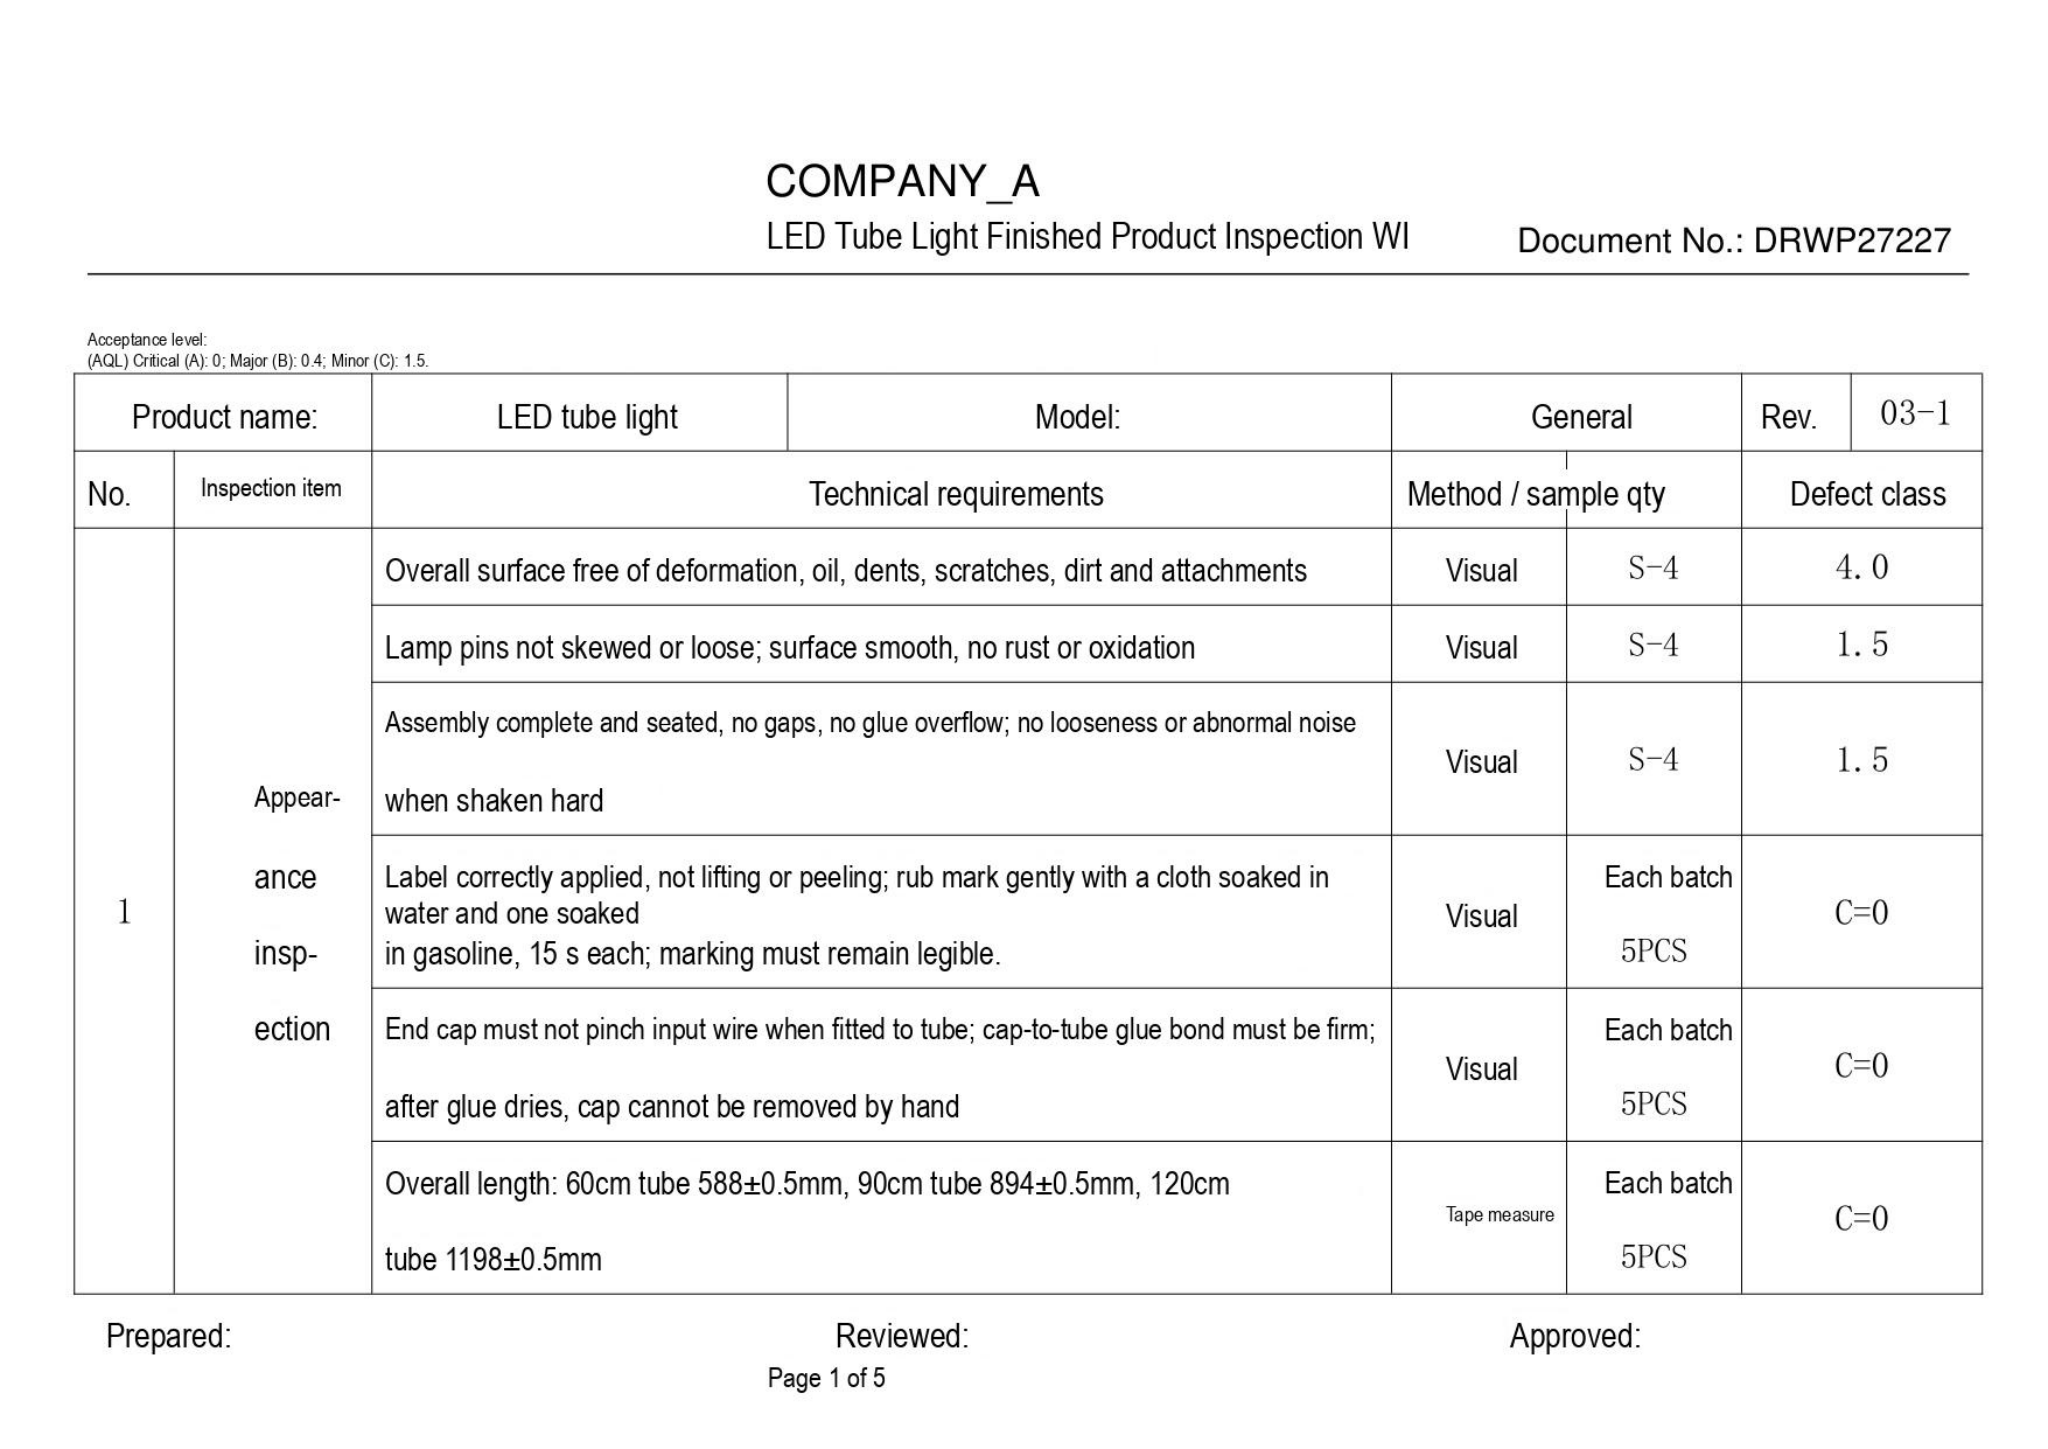COMPANY_A
LED Tube Light Finished Product Inspection WI
Document No.: DRWP27227

Acceptance level:
(AQL) Critical (A): 0; Major (B): 0.4; Minor (C): 1.5.

| Product name: | | LED tube light | Model: | General | | Rev. | 03-1 |
|---|---|---|---|---|---|---|---|
| No. | Inspection item | Technical requirements | | Method / sample qty | | Defect class | |
| 1 | Appear-ance insp-ection | Overall surface free of deformation, oil, dents, scratches, dirt and attachments | | Visual | S-4 | 4.0 | |
| | | Lamp pins not skewed or loose; surface smooth, no rust or oxidation | | Visual | S-4 | 1.5 | |
| | | Assembly complete and seated, no gaps, no glue overflow; no looseness or abnormal noise when shaken hard | | Visual | S-4 | 1.5 | |
| | | Label correctly applied, not lifting or peeling; rub mark gently with a cloth soaked in water and one soaked in gasoline, 15 s each; marking must remain legible. | | Visual | Each batch 5PCS | C=0 | |
| | | End cap must not pinch input wire when fitted to tube; cap-to-tube glue bond must be firm; after glue dries, cap cannot be removed by hand | | Visual | Each batch 5PCS | C=0 | |
| | | Overall length: 60cm tube 588±0.5mm, 90cm tube 894±0.5mm, 120cm tube 1198±0.5mm | | Tape measure | Each batch 5PCS | C=0 | |

Prepared: Reviewed: Approved:

Page 1 of 5
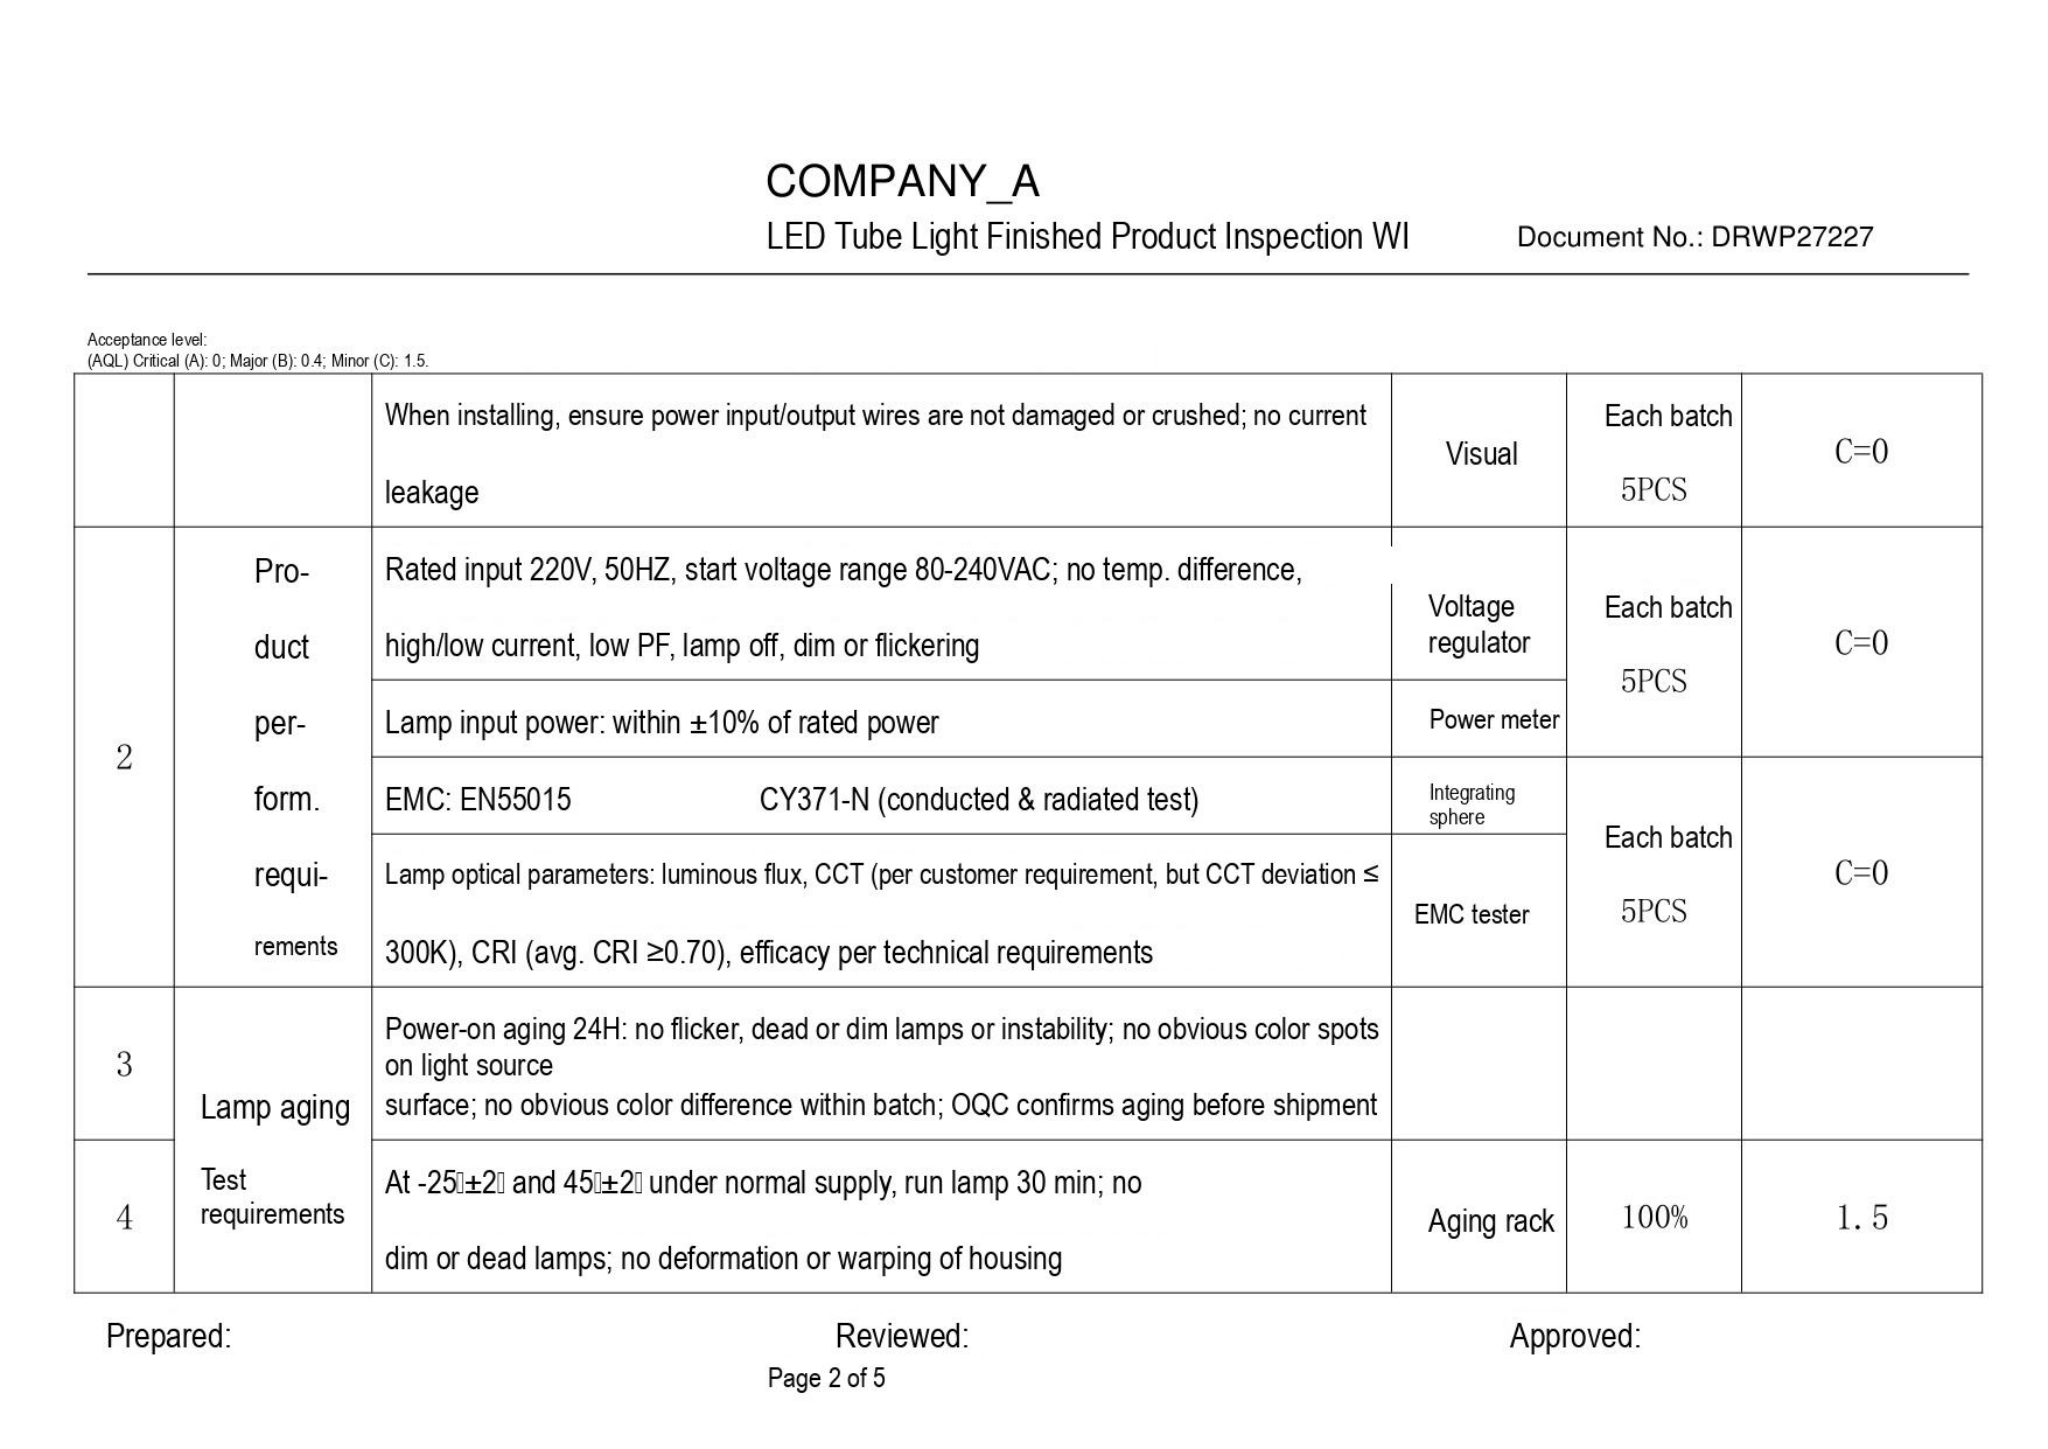COMPANY_A

LED Tube Light Finished Product Inspection WI　　Document No.: DRWP27227

Acceptance level:
(AQL) Critical (A): 0; Major (B): 0.4; Minor (C): 1.5.

| | | | | | |
|---|---|---|---|---|---|
| | | When installing, ensure power input/output wires are not damaged or crushed; no current leakage | Visual | Each batch 5PCS | C=0 |
| 2 | Pro- duct per- form. requi- rements | Rated input 220V, 50HZ, start voltage range 80-240VAC; no temp. difference, high/low current, low PF, lamp off, dim or flickering | Voltage regulator | Each batch 5PCS | C=0 |
| | | Lamp input power: within ±10% of rated power | Power meter | | |
| | | EMC: EN55015　　CY371-N (conducted & radiated test) | Integrating sphere | Each batch 5PCS | C=0 |
| | | Lamp optical parameters: luminous flux, CCT (per customer requirement, but CCT deviation ≤ 300K), CRI (avg. CRI ≥0.70), efficacy per technical requirements | EMC tester | | |
| 3 | Lamp aging | Power-on aging 24H: no flicker, dead or dim lamps or instability; no obvious color spots on light source surface; no obvious color difference within batch; OQC confirms aging before shipment | | | |
| 4 | Test requirements | At -25±2 and 45±2 under normal supply, run lamp 30 min; no dim or dead lamps; no deformation or warping of housing | Aging rack | 100% | 1.5 |

Prepared:　　Reviewed:　　Approved:

Page 2 of 5
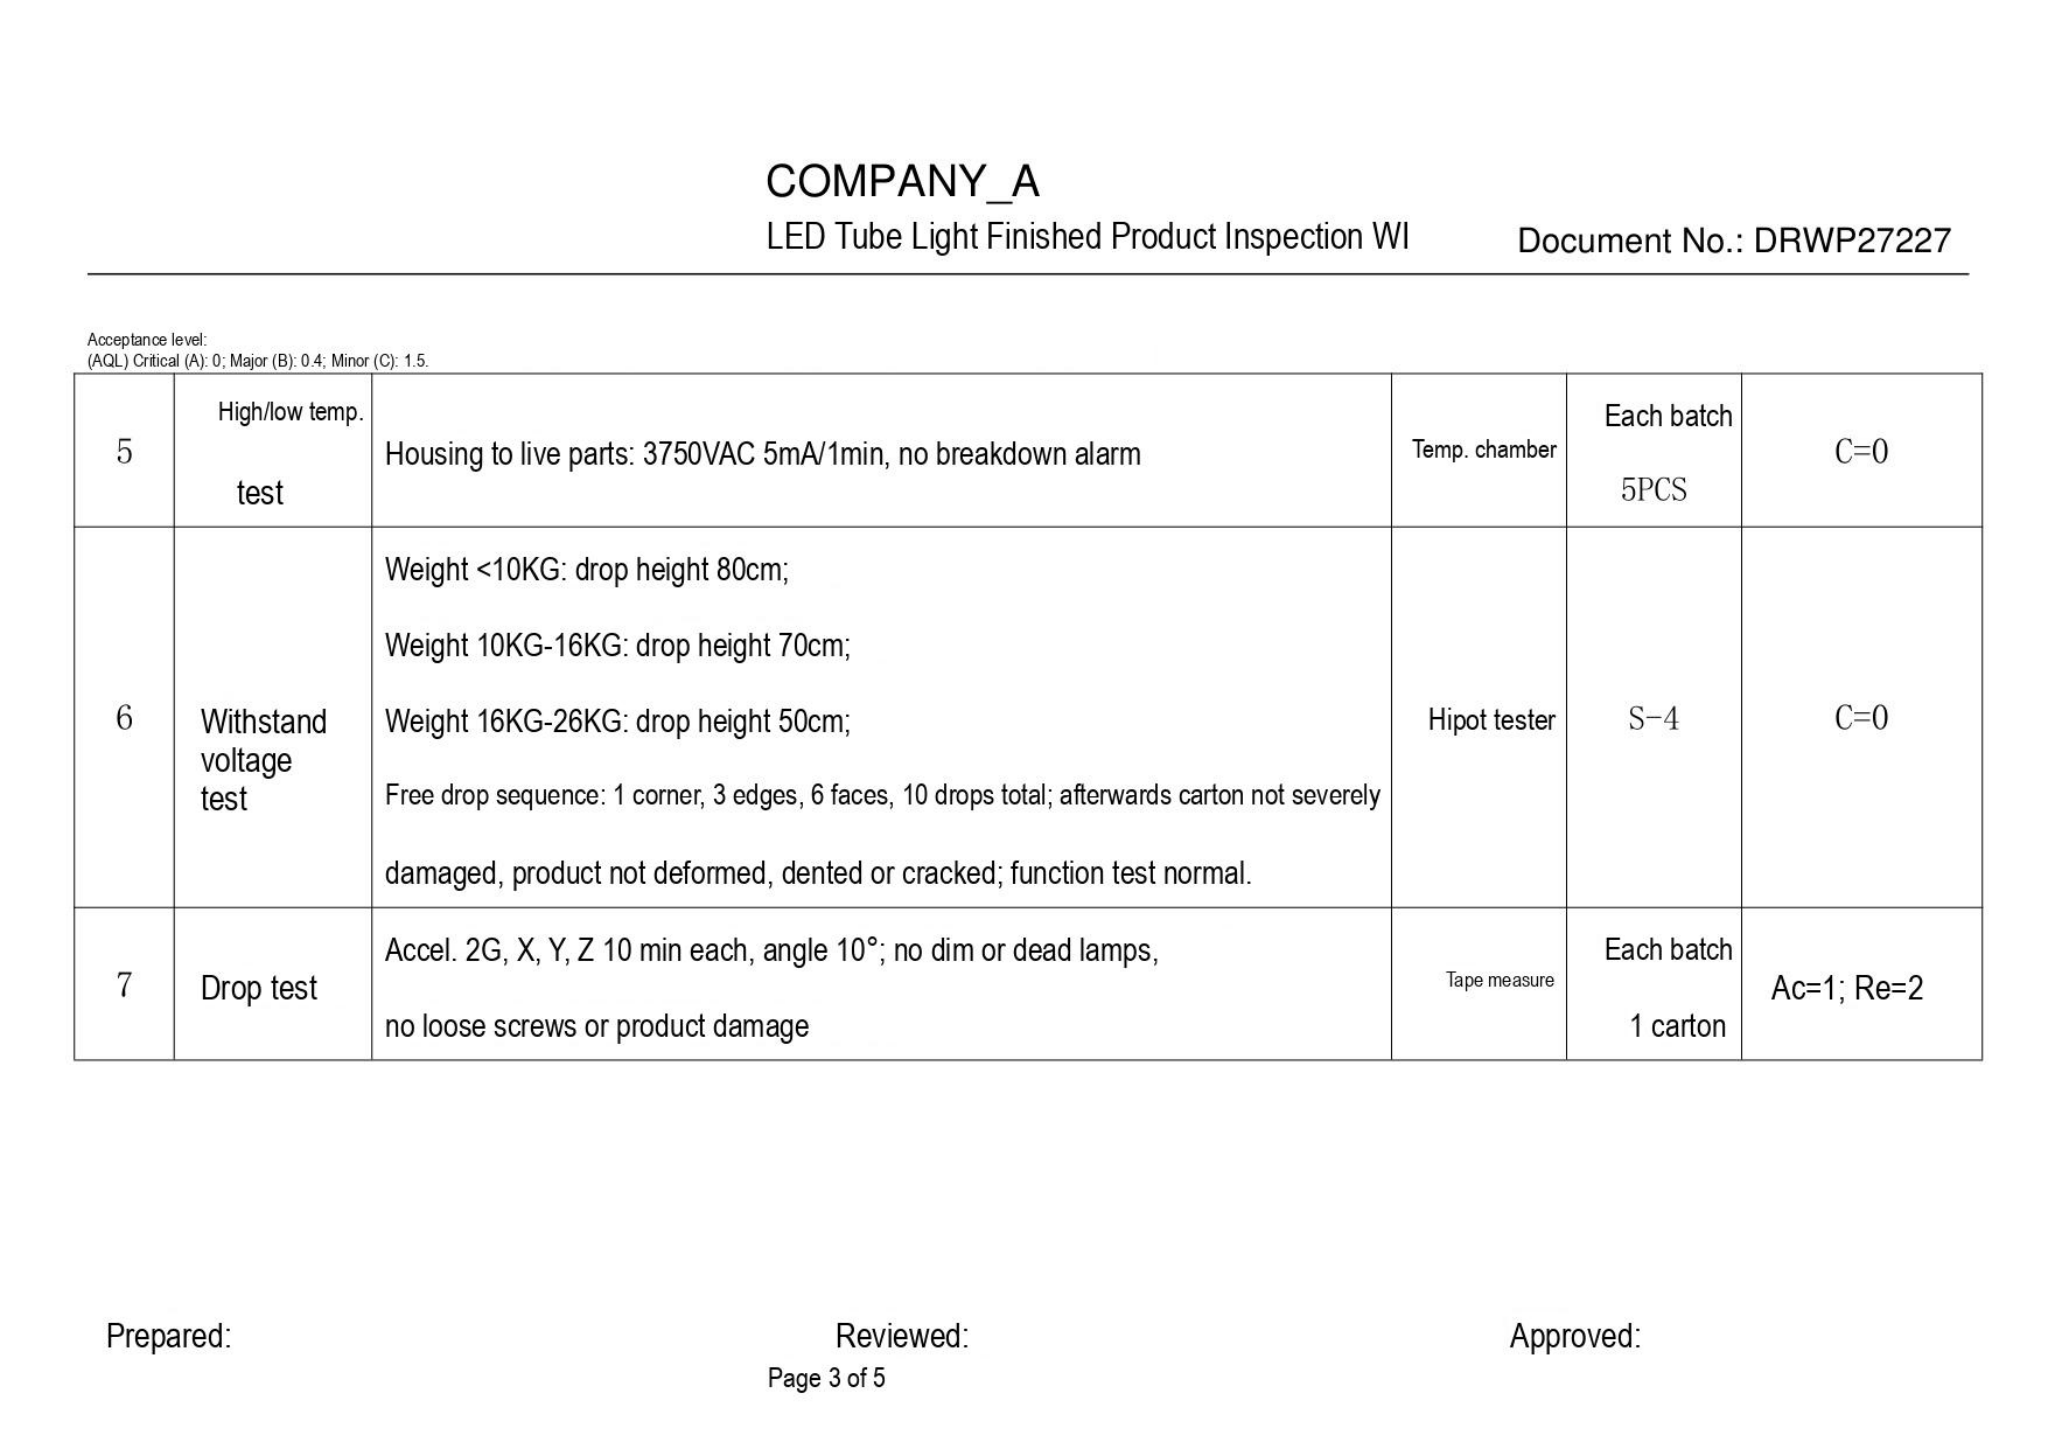COMPANY_A

LED Tube Light Finished Product Inspection WI

Document No.: DRWP27227

Acceptance level:
(AQL) Critical (A): 0; Major (B): 0.4; Minor (C): 1.5.

| 5 | High/low temp. test | Housing to live parts: 3750VAC 5mA/1min, no breakdown alarm | Temp. chamber | Each batch 5PCS | C=0 |
|---|---|---|---|---|---|
| 6 | Withstand voltage test | Weight <10KG: drop height 80cm; Weight 10KG-16KG: drop height 70cm; Weight 16KG-26KG: drop height 50cm; Free drop sequence: 1 corner, 3 edges, 6 faces, 10 drops total; afterwards carton not severely damaged, product not deformed, dented or cracked; function test normal. | Hipot tester | S-4 | C=0 |
| 7 | Drop test | Accel. 2G, X, Y, Z 10 min each, angle 10°; no dim or dead lamps, no loose screws or product damage | Tape measure | Each batch 1 carton | Ac=1; Re=2 |

Prepared:

Reviewed:

Approved:

Page 3 of 5
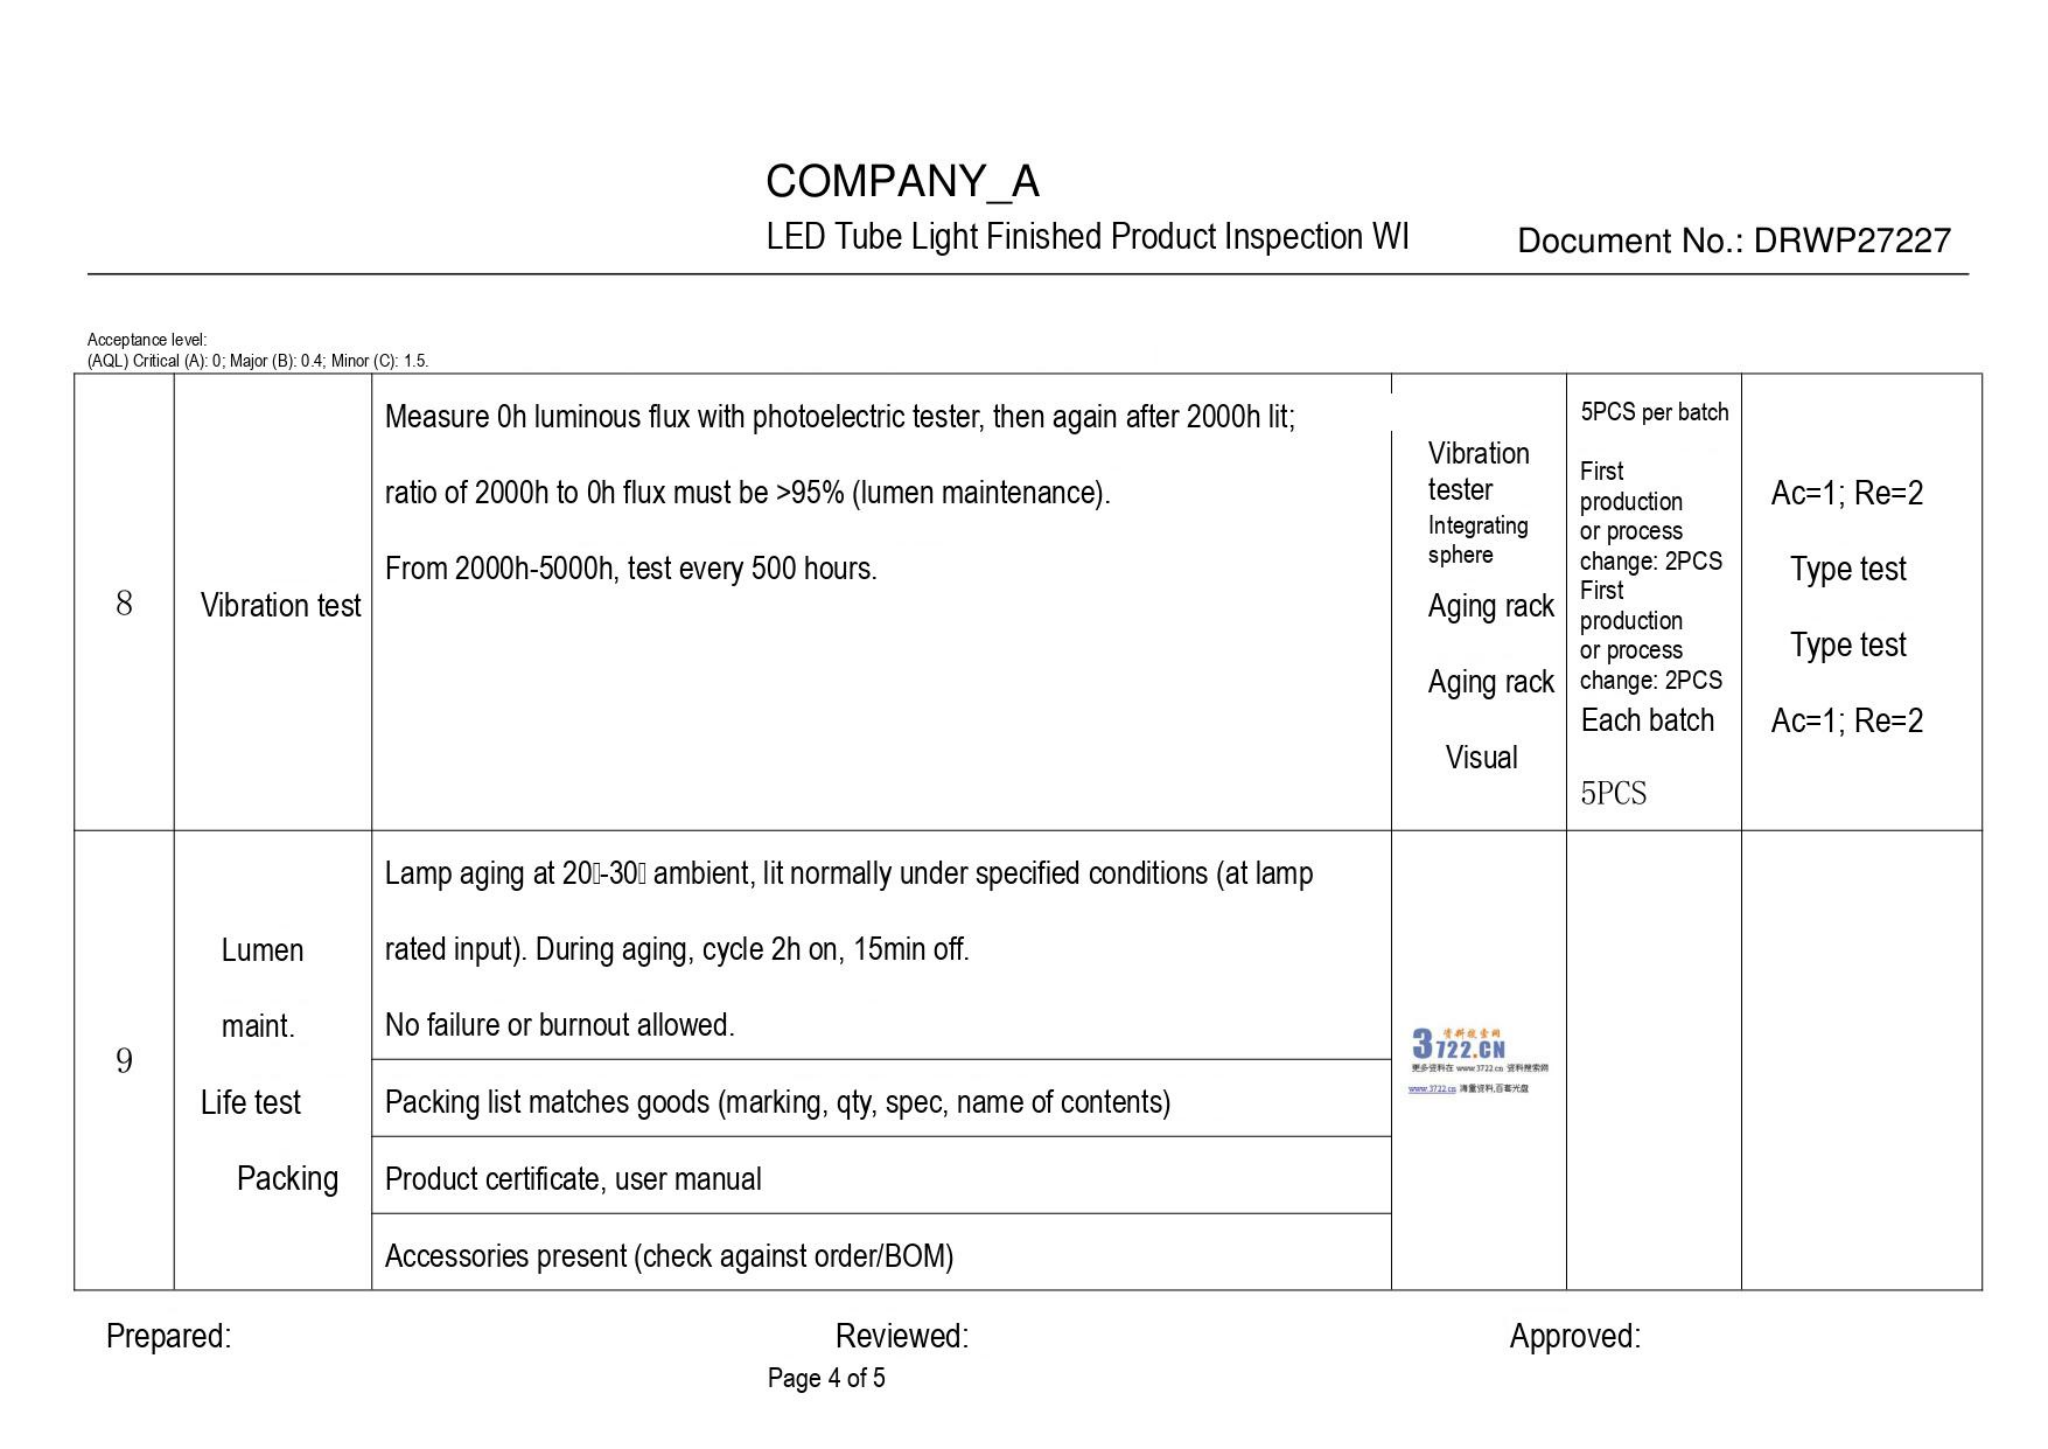COMPANY_A

LED Tube Light Finished Product Inspection WI

Document No.: DRWP27227

Acceptance level:
(AQL) Critical (A): 0; Major (B): 0.4; Minor (C): 1.5.

| | | | | | |
|---|---|---|---|---|---|
| 8 | Vibration test | Measure 0h luminous flux with photoelectric tester, then again after 2000h lit;<br>ratio of 2000h to 0h flux must be >95% (lumen maintenance).<br>From 2000h-5000h, test every 500 hours. | Vibration tester<br>Integrating sphere<br>Aging rack<br>Aging rack<br>Visual | 5PCS per batch<br>First production or process change: 2PCS<br>First production or process change: 2PCS<br>Each batch<br>5PCS | Ac=1; Re=2<br>Type test<br>Type test<br>Ac=1; Re=2 |
| 9 | Lumen maint.<br>Life test<br>Packing | Lamp aging at 20-30 ambient, lit normally under specified conditions (at lamp rated input). During aging, cycle 2h on, 15min off.<br>No failure or burnout allowed. | 3722.CN | | |
| | | Packing list matches goods (marking, qty, spec, name of contents) | | | |
| | | Product certificate, user manual | | | |
| | | Accessories present (check against order/BOM) | | | |

Prepared: Reviewed: Approved:

Page 4 of 5
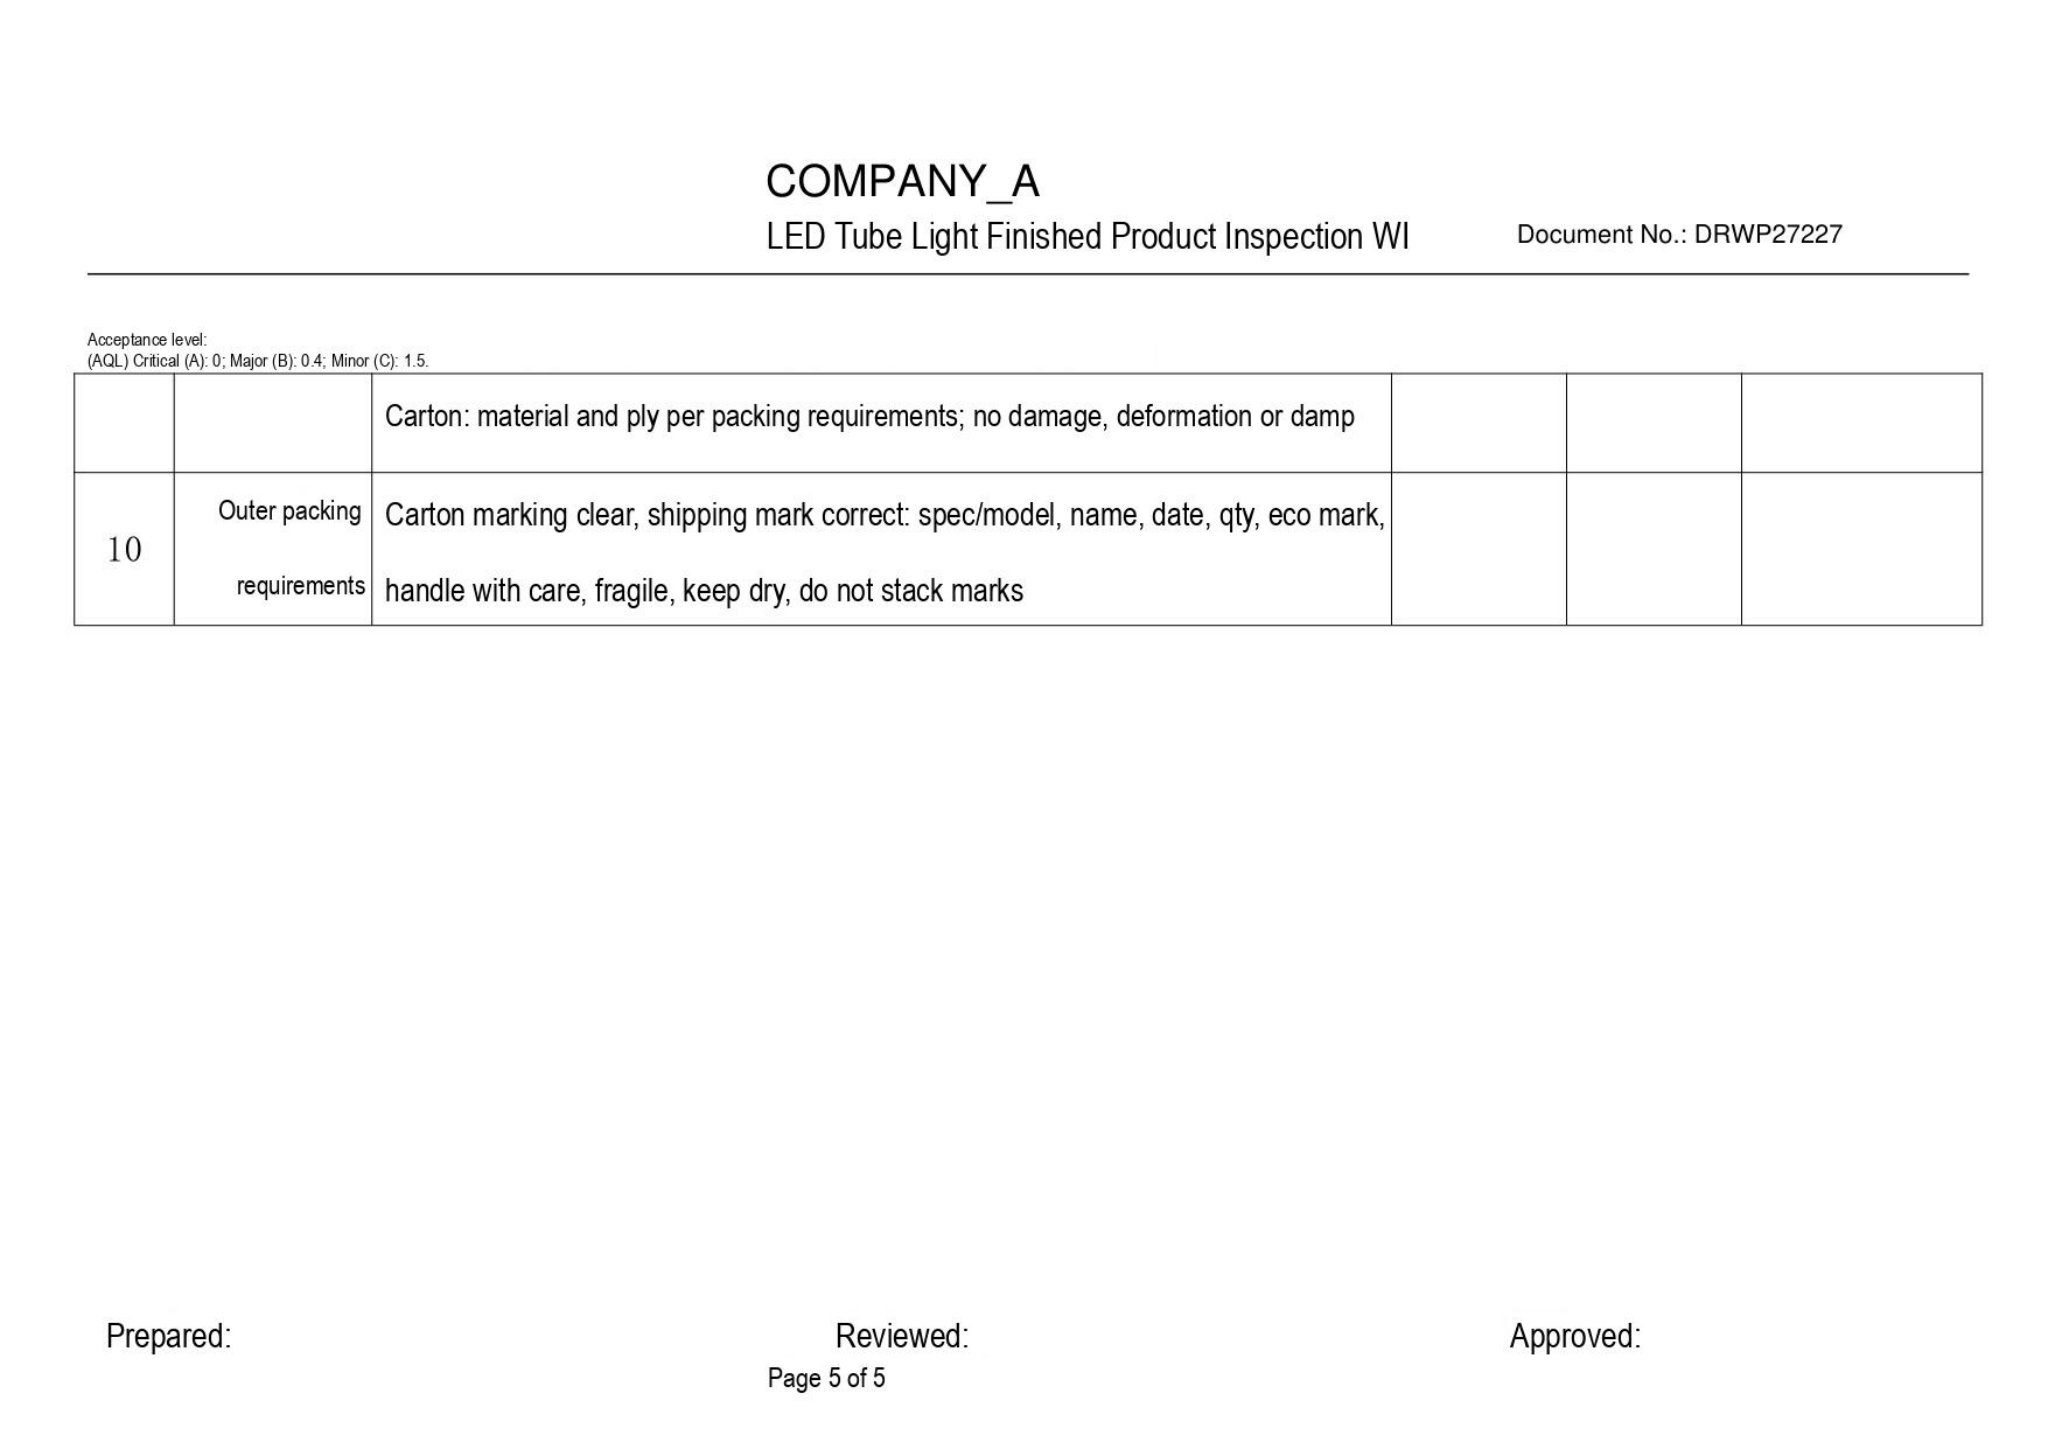COMPANY_A
LED Tube Light Finished Product Inspection WI
Document No.: DRWP27227

Acceptance level:
(AQL) Critical (A): 0; Major (B): 0.4; Minor (C): 1.5.

| | | | | | |
|---|---|---|---|---|---|
| | | Carton: material and ply per packing requirements; no damage, deformation or damp | | | |
| 10 | Outer packing requirements | Carton marking clear, shipping mark correct: spec/model, name, date, qty, eco mark, handle with care, fragile, keep dry, do not stack marks | | | |

Prepared:
Reviewed:
Approved:
Page 5 of 5